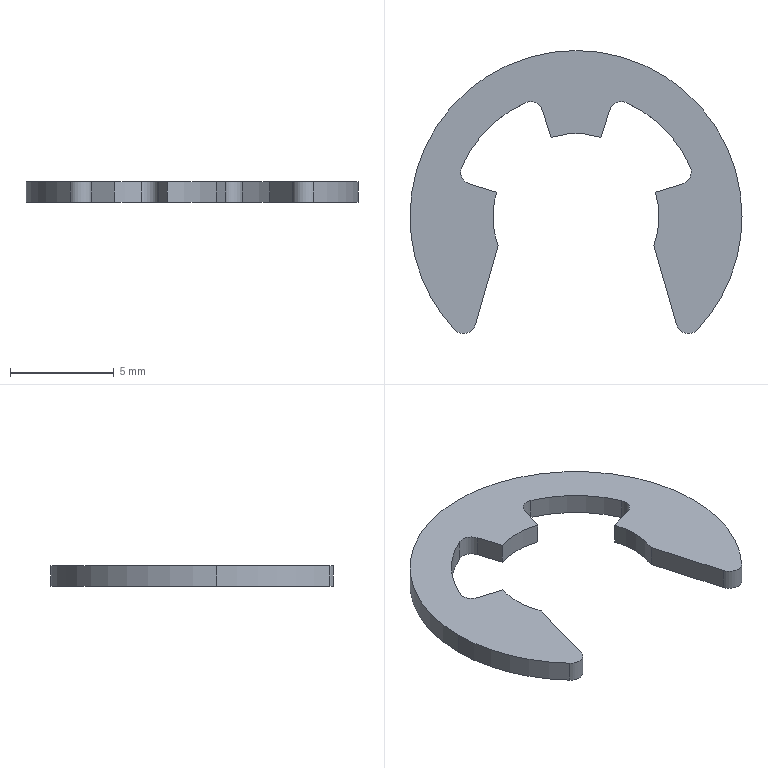Part | SolidWorks | features Extrusion 1 | 1 solid | 24 faces | box 16 x 13.638 x 1 mm | volume 90.427 mm3 | cylinder 16 | plane 8 | commonest cylinder face diameters 1.2 x7 8 x4 16 x3 12 x2
STEP:
#1=CARTESIAN_POINT('',(-5.507,2.381,1.));
#2=VERTEX_POINT('',#1);
#3=CARTESIAN_POINT('',(-5.557,2.143,1.));
#4=VERTEX_POINT('',#3);
#5=CARTESIAN_POINT('',(-4.957,2.143,1.));
#6=DIRECTION('',(0.,0.,1.));
#7=DIRECTION('',(1.,0.,0.));
#8=AXIS2_PLACEMENT_3D('',#5,#6,#7);
#9=CIRCLE('',#8,0.6);
#10=EDGE_CURVE('',#2,#4,#9,.T.);
#11=ORIENTED_EDGE('',*,*,#10,.T.);
#12=CARTESIAN_POINT('',(-5.557,2.143,0.));
#13=VERTEX_POINT('',#12);
#14=CARTESIAN_POINT('',(-5.557,2.143,1.));
#15=DIRECTION('',(0.,0.,-1.));
#16=VECTOR('',#15,1000.);
#17=LINE('',#14,#16);
#18=EDGE_CURVE('',#4,#13,#17,.T.);
#19=ORIENTED_EDGE('',*,*,#18,.T.);
#20=CARTESIAN_POINT('',(-5.507,2.381,0.));
#21=VERTEX_POINT('',#20);
#22=CARTESIAN_POINT('',(-4.957,2.143,0.));
#23=DIRECTION('',(0.,0.,1.));
#24=DIRECTION('',(1.,0.,0.));
#25=AXIS2_PLACEMENT_3D('',#22,#23,#24);
#26=CIRCLE('',#25,0.6);
#27=EDGE_CURVE('',#21,#13,#26,.T.);
#28=ORIENTED_EDGE('',*,*,#27,.F.);
#29=CARTESIAN_POINT('',(-5.507,2.381,1.));
#30=DIRECTION('',(0.,0.,-1.));
#31=VECTOR('',#30,1000.);
#32=LINE('',#29,#31);
#33=EDGE_CURVE('',#2,#21,#32,.T.);
#34=ORIENTED_EDGE('',*,*,#33,.F.);
#35=EDGE_LOOP('',(#11,#19,#28,#34));
#36=FACE_OUTER_BOUND('',#35,.T.);
#37=CARTESIAN_POINT('',(-4.957,2.143,1.));
#38=DIRECTION('',(0.,0.,-1.));
#39=DIRECTION('',(-1.,0.,0.));
#40=AXIS2_PLACEMENT_3D('',#37,#38,#39);
#41=CYLINDRICAL_SURFACE('',#40,0.6);
#42=ADVANCED_FACE('',(#36),#41,.F.);
#43=CARTESIAN_POINT('',(-3.825,1.169,1.));
#44=VERTEX_POINT('',#43);
#45=CARTESIAN_POINT('',(-4.,0.,1.));
#46=VERTEX_POINT('',#45);
#47=CARTESIAN_POINT('',(0.,0.,1.));
#48=DIRECTION('',(0.,0.,1.));
#49=DIRECTION('',(1.,0.,0.));
#50=AXIS2_PLACEMENT_3D('',#47,#48,#49);
#51=CIRCLE('',#50,4.);
#52=EDGE_CURVE('',#44,#46,#51,.T.);
#53=ORIENTED_EDGE('',*,*,#52,.T.);
#54=CARTESIAN_POINT('',(-4.,0.,0.));
#55=VERTEX_POINT('',#54);
#56=CARTESIAN_POINT('',(-4.,0.,1.));
#57=DIRECTION('',(0.,0.,-1.));
#58=VECTOR('',#57,1000.);
#59=LINE('',#56,#58);
#60=EDGE_CURVE('',#46,#55,#59,.T.);
#61=ORIENTED_EDGE('',*,*,#60,.T.);
#62=CARTESIAN_POINT('',(-3.825,1.169,0.));
#63=VERTEX_POINT('',#62);
#64=CARTESIAN_POINT('',(0.,0.,0.));
#65=DIRECTION('',(0.,0.,1.));
#66=DIRECTION('',(1.,0.,0.));
#67=AXIS2_PLACEMENT_3D('',#64,#65,#66);
#68=CIRCLE('',#67,4.);
#69=EDGE_CURVE('',#63,#55,#68,.T.);
#70=ORIENTED_EDGE('',*,*,#69,.F.);
#71=CARTESIAN_POINT('',(-3.825,1.169,1.));
#72=DIRECTION('',(0.,0.,-1.));
#73=VECTOR('',#72,1000.);
#74=LINE('',#71,#73);
#75=EDGE_CURVE('',#44,#63,#74,.T.);
#76=ORIENTED_EDGE('',*,*,#75,.F.);
#77=EDGE_LOOP('',(#53,#61,#70,#76));
#78=FACE_OUTER_BOUND('',#77,.T.);
#79=CARTESIAN_POINT('',(0.,0.,1.));
#80=DIRECTION('',(0.,0.,-1.));
#81=DIRECTION('',(-1.,0.,0.));
#82=AXIS2_PLACEMENT_3D('',#79,#80,#81);
#83=CYLINDRICAL_SURFACE('',#82,4.);
#84=ADVANCED_FACE('',(#78),#83,.F.);
#85=CARTESIAN_POINT('',(8.,0.,1.));
#86=VERTEX_POINT('',#85);
#87=CARTESIAN_POINT('',(-8.,0.,1.));
#88=VERTEX_POINT('',#87);
#89=CARTESIAN_POINT('',(0.,0.,1.));
#90=DIRECTION('',(0.,0.,1.));
#91=DIRECTION('',(1.,0.,0.));
#92=AXIS2_PLACEMENT_3D('',#89,#90,#91);
#93=CIRCLE('',#92,8.);
#94=EDGE_CURVE('',#86,#88,#93,.T.);
#95=ORIENTED_EDGE('',*,*,#94,.F.);
#96=CARTESIAN_POINT('',(8.,0.,0.));
#97=VERTEX_POINT('',#96);
#98=CARTESIAN_POINT('',(8.,0.,1.));
#99=DIRECTION('',(0.,0.,-1.));
#100=VECTOR('',#99,1000.);
#101=LINE('',#98,#100);
#102=EDGE_CURVE('',#86,#97,#101,.T.);
#103=ORIENTED_EDGE('',*,*,#102,.T.);
#104=CARTESIAN_POINT('',(-8.,0.,0.));
#105=VERTEX_POINT('',#104);
#106=CARTESIAN_POINT('',(0.,0.,0.));
#107=DIRECTION('',(0.,0.,1.));
#108=DIRECTION('',(1.,0.,0.));
#109=AXIS2_PLACEMENT_3D('',#106,#107,#108);
#110=CIRCLE('',#109,8.);
#111=EDGE_CURVE('',#97,#105,#110,.T.);
#112=ORIENTED_EDGE('',*,*,#111,.T.);
#113=CARTESIAN_POINT('',(-8.,0.,1.));
#114=DIRECTION('',(0.,0.,-1.));
#115=VECTOR('',#114,1000.);
#116=LINE('',#113,#115);
#117=EDGE_CURVE('',#88,#105,#116,.T.);
#118=ORIENTED_EDGE('',*,*,#117,.F.);
#119=EDGE_LOOP('',(#95,#103,#112,#118));
#120=FACE_OUTER_BOUND('',#119,.T.);
#121=CARTESIAN_POINT('',(0.,0.,1.));
#122=DIRECTION('',(0.,0.,-1.));
#123=DIRECTION('',(-1.,0.,0.));
#124=AXIS2_PLACEMENT_3D('',#121,#122,#123);
#125=CYLINDRICAL_SURFACE('',#124,8.);
#126=ADVANCED_FACE('',(#120),#125,.T.);
#127=CARTESIAN_POINT('',(-5.859,-5.447,1.));
#128=VERTEX_POINT('',#127);
#129=CARTESIAN_POINT('',(0.,0.,1.));
#130=DIRECTION('',(0.,0.,1.));
#131=DIRECTION('',(1.,0.,0.));
#132=AXIS2_PLACEMENT_3D('',#129,#130,#131);
#133=CIRCLE('',#132,8.);
#134=EDGE_CURVE('',#88,#128,#133,.T.);
#135=ORIENTED_EDGE('',*,*,#134,.F.);
#136=ORIENTED_EDGE('',*,*,#117,.T.);
#137=CARTESIAN_POINT('',(-5.859,-5.447,0.));
#138=VERTEX_POINT('',#137);
#139=CARTESIAN_POINT('',(0.,0.,0.));
#140=DIRECTION('',(0.,0.,1.));
#141=DIRECTION('',(1.,0.,0.));
#142=AXIS2_PLACEMENT_3D('',#139,#140,#141);
#143=CIRCLE('',#142,8.);
#144=EDGE_CURVE('',#105,#138,#143,.T.);
#145=ORIENTED_EDGE('',*,*,#144,.T.);
#146=CARTESIAN_POINT('',(-5.859,-5.447,1.));
#147=DIRECTION('',(0.,0.,-1.));
#148=VECTOR('',#147,1000.);
#149=LINE('',#146,#148);
#150=EDGE_CURVE('',#128,#138,#149,.T.);
#151=ORIENTED_EDGE('',*,*,#150,.F.);
#152=EDGE_LOOP('',(#135,#136,#145,#151));
#153=FACE_OUTER_BOUND('',#152,.T.);
#154=CARTESIAN_POINT('',(0.,0.,1.));
#155=DIRECTION('',(0.,0.,-1.));
#156=DIRECTION('',(-1.,0.,0.));
#157=AXIS2_PLACEMENT_3D('',#154,#155,#156);
#158=CYLINDRICAL_SURFACE('',#157,8.);
#159=ADVANCED_FACE('',(#153),#158,.T.);
#160=CARTESIAN_POINT('',(5.507,2.381,0.));
#161=VERTEX_POINT('',#160);
#162=CARTESIAN_POINT('',(2.429,5.486,0.));
#163=VERTEX_POINT('',#162);
#164=CARTESIAN_POINT('',(0.,0.,0.));
#165=DIRECTION('',(0.,0.,1.));
#166=DIRECTION('',(1.,0.,0.));
#167=AXIS2_PLACEMENT_3D('',#164,#165,#166);
#168=CIRCLE('',#167,6.);
#169=EDGE_CURVE('',#161,#163,#168,.T.);
#170=ORIENTED_EDGE('',*,*,#169,.F.);
#171=CARTESIAN_POINT('',(5.507,2.381,1.));
#172=VERTEX_POINT('',#171);
#173=CARTESIAN_POINT('',(5.507,2.381,1.));
#174=DIRECTION('',(0.,0.,-1.));
#175=VECTOR('',#174,1000.);
#176=LINE('',#173,#175);
#177=EDGE_CURVE('',#172,#161,#176,.T.);
#178=ORIENTED_EDGE('',*,*,#177,.F.);
#179=CARTESIAN_POINT('',(2.429,5.486,1.));
#180=VERTEX_POINT('',#179);
#181=CARTESIAN_POINT('',(0.,0.,1.));
#182=DIRECTION('',(0.,0.,1.));
#183=DIRECTION('',(1.,0.,0.));
#184=AXIS2_PLACEMENT_3D('',#181,#182,#183);
#185=CIRCLE('',#184,6.);
#186=EDGE_CURVE('',#172,#180,#185,.T.);
#187=ORIENTED_EDGE('',*,*,#186,.T.);
#188=CARTESIAN_POINT('',(2.429,5.486,1.));
#189=DIRECTION('',(0.,0.,-1.));
#190=VECTOR('',#189,1000.);
#191=LINE('',#188,#190);
#192=EDGE_CURVE('',#180,#163,#191,.T.);
#193=ORIENTED_EDGE('',*,*,#192,.T.);
#194=EDGE_LOOP('',(#170,#178,#187,#193));
#195=FACE_OUTER_BOUND('',#194,.T.);
#196=CARTESIAN_POINT('',(0.,0.,1.));
#197=DIRECTION('',(0.,0.,-1.));
#198=DIRECTION('',(-1.,0.,0.));
#199=AXIS2_PLACEMENT_3D('',#196,#197,#198);
#200=CYLINDRICAL_SURFACE('',#199,6.);
#201=ADVANCED_FACE('',(#195),#200,.F.);
#202=CARTESIAN_POINT('',(5.132,1.569,0.));
#203=VERTEX_POINT('',#202);
#204=CARTESIAN_POINT('',(4.957,2.143,0.));
#205=DIRECTION('',(0.,0.,-1.));
#206=DIRECTION('',(1.,0.,0.));
#207=AXIS2_PLACEMENT_3D('',#204,#205,#206);
#208=CIRCLE('',#207,0.6);
#209=EDGE_CURVE('',#161,#203,#208,.T.);
#210=ORIENTED_EDGE('',*,*,#209,.T.);
#211=CARTESIAN_POINT('',(5.132,1.569,1.));
#212=VERTEX_POINT('',#211);
#213=CARTESIAN_POINT('',(5.132,1.569,1.));
#214=DIRECTION('',(0.,0.,-1.));
#215=VECTOR('',#214,1000.);
#216=LINE('',#213,#215);
#217=EDGE_CURVE('',#212,#203,#216,.T.);
#218=ORIENTED_EDGE('',*,*,#217,.F.);
#219=CARTESIAN_POINT('',(4.957,2.143,1.));
#220=DIRECTION('',(0.,0.,-1.));
#221=DIRECTION('',(1.,0.,0.));
#222=AXIS2_PLACEMENT_3D('',#219,#220,#221);
#223=CIRCLE('',#222,0.6);
#224=EDGE_CURVE('',#172,#212,#223,.T.);
#225=ORIENTED_EDGE('',*,*,#224,.F.);
#226=ORIENTED_EDGE('',*,*,#177,.T.);
#227=EDGE_LOOP('',(#210,#218,#225,#226));
#228=FACE_OUTER_BOUND('',#227,.T.);
#229=CARTESIAN_POINT('',(4.957,2.143,1.));
#230=DIRECTION('',(0.,0.,-1.));
#231=DIRECTION('',(-1.,0.,0.));
#232=AXIS2_PLACEMENT_3D('',#229,#230,#231);
#233=CYLINDRICAL_SURFACE('',#232,0.6);
#234=ADVANCED_FACE('',(#228),#233,.F.);
#235=CARTESIAN_POINT('',(3.825,1.169,0.));
#236=VERTEX_POINT('',#235);
#237=CARTESIAN_POINT('',(0.,0.,0.));
#238=DIRECTION('',(0.9563,0.2924,0.));
#239=VECTOR('',#238,1000.);
#240=LINE('',#237,#239);
#241=EDGE_CURVE('',#236,#203,#240,.T.);
#242=ORIENTED_EDGE('',*,*,#241,.F.);
#243=CARTESIAN_POINT('',(3.825,1.169,1.));
#244=VERTEX_POINT('',#243);
#245=CARTESIAN_POINT('',(3.825,1.169,1.));
#246=DIRECTION('',(0.,0.,-1.));
#247=VECTOR('',#246,1000.);
#248=LINE('',#245,#247);
#249=EDGE_CURVE('',#244,#236,#248,.T.);
#250=ORIENTED_EDGE('',*,*,#249,.F.);
#251=CARTESIAN_POINT('',(0.,0.,1.));
#252=DIRECTION('',(0.9563,0.2924,0.));
#253=VECTOR('',#252,1000.);
#254=LINE('',#251,#253);
#255=EDGE_CURVE('',#244,#212,#254,.T.);
#256=ORIENTED_EDGE('',*,*,#255,.T.);
#257=ORIENTED_EDGE('',*,*,#217,.T.);
#258=EDGE_LOOP('',(#242,#250,#256,#257));
#259=FACE_OUTER_BOUND('',#258,.T.);
#260=CARTESIAN_POINT('',(0.,0.,1.));
#261=DIRECTION('',(-0.2924,0.9563,0.));
#262=DIRECTION('',(-0.9563,-0.2924,0.));
#263=AXIS2_PLACEMENT_3D('',#260,#261,#262);
#264=PLANE('',#263);
#265=ADVANCED_FACE('',(#259),#264,.T.);
#266=CARTESIAN_POINT('',(3.75,-1.392,0.));
#267=VERTEX_POINT('',#266);
#268=CARTESIAN_POINT('',(0.,0.,0.));
#269=DIRECTION('',(0.,0.,1.));
#270=DIRECTION('',(1.,0.,0.));
#271=AXIS2_PLACEMENT_3D('',#268,#269,#270);
#272=CIRCLE('',#271,4.);
#273=EDGE_CURVE('',#267,#236,#272,.T.);
#274=ORIENTED_EDGE('',*,*,#273,.F.);
#275=CARTESIAN_POINT('',(3.75,-1.392,1.));
#276=VERTEX_POINT('',#275);
#277=CARTESIAN_POINT('',(3.75,-1.392,1.));
#278=DIRECTION('',(0.,0.,-1.));
#279=VECTOR('',#278,1000.);
#280=LINE('',#277,#279);
#281=EDGE_CURVE('',#276,#267,#280,.T.);
#282=ORIENTED_EDGE('',*,*,#281,.F.);
#283=CARTESIAN_POINT('',(0.,0.,1.));
#284=DIRECTION('',(0.,0.,1.));
#285=DIRECTION('',(1.,0.,0.));
#286=AXIS2_PLACEMENT_3D('',#283,#284,#285);
#287=CIRCLE('',#286,4.);
#288=EDGE_CURVE('',#276,#244,#287,.T.);
#289=ORIENTED_EDGE('',*,*,#288,.T.);
#290=ORIENTED_EDGE('',*,*,#249,.T.);
#291=EDGE_LOOP('',(#274,#282,#289,#290));
#292=FACE_OUTER_BOUND('',#291,.T.);
#293=CARTESIAN_POINT('',(0.,0.,1.));
#294=DIRECTION('',(0.,0.,-1.));
#295=DIRECTION('',(-1.,0.,0.));
#296=AXIS2_PLACEMENT_3D('',#293,#294,#295);
#297=CYLINDRICAL_SURFACE('',#296,4.);
#298=ADVANCED_FACE('',(#292),#297,.F.);
#299=CARTESIAN_POINT('',(4.843,-5.204,0.));
#300=VERTEX_POINT('',#299);
#301=CARTESIAN_POINT('',(3.096,0.8878,0.));
#302=DIRECTION('',(0.2756,-0.9613,0.));
#303=VECTOR('',#302,1000.);
#304=LINE('',#301,#303);
#305=EDGE_CURVE('',#267,#300,#304,.T.);
#306=ORIENTED_EDGE('',*,*,#305,.T.);
#307=CARTESIAN_POINT('',(4.843,-5.204,1.));
#308=VERTEX_POINT('',#307);
#309=CARTESIAN_POINT('',(4.843,-5.204,1.));
#310=DIRECTION('',(0.,0.,-1.));
#311=VECTOR('',#310,1000.);
#312=LINE('',#309,#311);
#313=EDGE_CURVE('',#308,#300,#312,.T.);
#314=ORIENTED_EDGE('',*,*,#313,.F.);
#315=CARTESIAN_POINT('',(3.096,0.8878,1.));
#316=DIRECTION('',(0.2756,-0.9613,0.));
#317=VECTOR('',#316,1000.);
#318=LINE('',#315,#317);
#319=EDGE_CURVE('',#276,#308,#318,.T.);
#320=ORIENTED_EDGE('',*,*,#319,.F.);
#321=ORIENTED_EDGE('',*,*,#281,.T.);
#322=EDGE_LOOP('',(#306,#314,#320,#321));
#323=FACE_OUTER_BOUND('',#322,.T.);
#324=CARTESIAN_POINT('',(3.096,0.8878,1.));
#325=DIRECTION('',(0.9613,0.2756,0.));
#326=DIRECTION('',(-0.2756,0.9613,0.));
#327=AXIS2_PLACEMENT_3D('',#324,#325,#326);
#328=PLANE('',#327);
#329=ADVANCED_FACE('',(#323),#328,.F.);
#330=CARTESIAN_POINT('',(5.859,-5.447,0.));
#331=VERTEX_POINT('',#330);
#332=CARTESIAN_POINT('',(5.42,-5.038,0.));
#333=DIRECTION('',(0.,0.,-1.));
#334=DIRECTION('',(1.,0.,0.));
#335=AXIS2_PLACEMENT_3D('',#332,#333,#334);
#336=CIRCLE('',#335,0.6);
#337=EDGE_CURVE('',#331,#300,#336,.T.);
#338=ORIENTED_EDGE('',*,*,#337,.F.);
#339=CARTESIAN_POINT('',(5.859,-5.447,1.));
#340=VERTEX_POINT('',#339);
#341=CARTESIAN_POINT('',(5.859,-5.447,1.));
#342=DIRECTION('',(0.,0.,-1.));
#343=VECTOR('',#342,1000.);
#344=LINE('',#341,#343);
#345=EDGE_CURVE('',#340,#331,#344,.T.);
#346=ORIENTED_EDGE('',*,*,#345,.F.);
#347=CARTESIAN_POINT('',(5.42,-5.038,1.));
#348=DIRECTION('',(0.,0.,-1.));
#349=DIRECTION('',(1.,0.,0.));
#350=AXIS2_PLACEMENT_3D('',#347,#348,#349);
#351=CIRCLE('',#350,0.6);
#352=EDGE_CURVE('',#340,#308,#351,.T.);
#353=ORIENTED_EDGE('',*,*,#352,.T.);
#354=ORIENTED_EDGE('',*,*,#313,.T.);
#355=EDGE_LOOP('',(#338,#346,#353,#354));
#356=FACE_OUTER_BOUND('',#355,.T.);
#357=CARTESIAN_POINT('',(5.42,-5.038,1.));
#358=DIRECTION('',(0.,0.,-1.));
#359=DIRECTION('',(-1.,0.,0.));
#360=AXIS2_PLACEMENT_3D('',#357,#358,#359);
#361=CYLINDRICAL_SURFACE('',#360,0.6);
#362=ADVANCED_FACE('',(#356),#361,.T.);
#363=ORIENTED_EDGE('',*,*,#102,.F.);
#364=CARTESIAN_POINT('',(0.,0.,1.));
#365=DIRECTION('',(0.,0.,1.));
#366=DIRECTION('',(1.,0.,0.));
#367=AXIS2_PLACEMENT_3D('',#364,#365,#366);
#368=CIRCLE('',#367,8.);
#369=EDGE_CURVE('',#340,#86,#368,.T.);
#370=ORIENTED_EDGE('',*,*,#369,.F.);
#371=ORIENTED_EDGE('',*,*,#345,.T.);
#372=CARTESIAN_POINT('',(0.,0.,0.));
#373=DIRECTION('',(0.,0.,1.));
#374=DIRECTION('',(1.,0.,0.));
#375=AXIS2_PLACEMENT_3D('',#372,#373,#374);
#376=CIRCLE('',#375,8.);
#377=EDGE_CURVE('',#331,#97,#376,.T.);
#378=ORIENTED_EDGE('',*,*,#377,.T.);
#379=EDGE_LOOP('',(#363,#370,#371,#378));
#380=FACE_OUTER_BOUND('',#379,.T.);
#381=CARTESIAN_POINT('',(0.,0.,1.));
#382=DIRECTION('',(0.,0.,-1.));
#383=DIRECTION('',(-1.,0.,0.));
#384=AXIS2_PLACEMENT_3D('',#381,#382,#383);
#385=CYLINDRICAL_SURFACE('',#384,8.);
#386=ADVANCED_FACE('',(#380),#385,.T.);
#387=CARTESIAN_POINT('',(-4.843,-5.204,0.));
#388=VERTEX_POINT('',#387);
#389=CARTESIAN_POINT('',(-5.42,-5.038,0.));
#390=DIRECTION('',(0.,0.,-1.));
#391=DIRECTION('',(1.,0.,0.));
#392=AXIS2_PLACEMENT_3D('',#389,#390,#391);
#393=CIRCLE('',#392,0.6);
#394=EDGE_CURVE('',#388,#138,#393,.T.);
#395=ORIENTED_EDGE('',*,*,#394,.F.);
#396=CARTESIAN_POINT('',(-4.843,-5.204,1.));
#397=VERTEX_POINT('',#396);
#398=CARTESIAN_POINT('',(-4.843,-5.204,1.));
#399=DIRECTION('',(0.,0.,-1.));
#400=VECTOR('',#399,1000.);
#401=LINE('',#398,#400);
#402=EDGE_CURVE('',#397,#388,#401,.T.);
#403=ORIENTED_EDGE('',*,*,#402,.F.);
#404=CARTESIAN_POINT('',(-5.42,-5.038,1.));
#405=DIRECTION('',(0.,0.,-1.));
#406=DIRECTION('',(1.,0.,0.));
#407=AXIS2_PLACEMENT_3D('',#404,#405,#406);
#408=CIRCLE('',#407,0.6);
#409=EDGE_CURVE('',#397,#128,#408,.T.);
#410=ORIENTED_EDGE('',*,*,#409,.T.);
#411=ORIENTED_EDGE('',*,*,#150,.T.);
#412=EDGE_LOOP('',(#395,#403,#410,#411));
#413=FACE_OUTER_BOUND('',#412,.T.);
#414=CARTESIAN_POINT('',(-5.42,-5.038,1.));
#415=DIRECTION('',(0.,0.,-1.));
#416=DIRECTION('',(-1.,0.,0.));
#417=AXIS2_PLACEMENT_3D('',#414,#415,#416);
#418=CYLINDRICAL_SURFACE('',#417,0.6);
#419=ADVANCED_FACE('',(#413),#418,.T.);
#420=CARTESIAN_POINT('',(-3.75,-1.392,0.));
#421=VERTEX_POINT('',#420);
#422=CARTESIAN_POINT('',(-3.096,0.8878,0.));
#423=DIRECTION('',(-0.2756,-0.9613,0.));
#424=VECTOR('',#423,1000.);
#425=LINE('',#422,#424);
#426=EDGE_CURVE('',#421,#388,#425,.T.);
#427=ORIENTED_EDGE('',*,*,#426,.F.);
#428=CARTESIAN_POINT('',(-3.75,-1.392,1.));
#429=VERTEX_POINT('',#428);
#430=CARTESIAN_POINT('',(-3.75,-1.392,1.));
#431=DIRECTION('',(0.,0.,-1.));
#432=VECTOR('',#431,1000.);
#433=LINE('',#430,#432);
#434=EDGE_CURVE('',#429,#421,#433,.T.);
#435=ORIENTED_EDGE('',*,*,#434,.F.);
#436=CARTESIAN_POINT('',(-3.096,0.8878,1.));
#437=DIRECTION('',(-0.2756,-0.9613,0.));
#438=VECTOR('',#437,1000.);
#439=LINE('',#436,#438);
#440=EDGE_CURVE('',#429,#397,#439,.T.);
#441=ORIENTED_EDGE('',*,*,#440,.T.);
#442=ORIENTED_EDGE('',*,*,#402,.T.);
#443=EDGE_LOOP('',(#427,#435,#441,#442));
#444=FACE_OUTER_BOUND('',#443,.T.);
#445=CARTESIAN_POINT('',(-3.096,0.8878,1.));
#446=DIRECTION('',(0.9613,-0.2756,0.));
#447=DIRECTION('',(0.2756,0.9613,0.));
#448=AXIS2_PLACEMENT_3D('',#445,#446,#447);
#449=PLANE('',#448);
#450=ADVANCED_FACE('',(#444),#449,.T.);
#451=ORIENTED_EDGE('',*,*,#60,.F.);
#452=CARTESIAN_POINT('',(0.,0.,1.));
#453=DIRECTION('',(0.,0.,1.));
#454=DIRECTION('',(1.,0.,0.));
#455=AXIS2_PLACEMENT_3D('',#452,#453,#454);
#456=CIRCLE('',#455,4.);
#457=EDGE_CURVE('',#46,#429,#456,.T.);
#458=ORIENTED_EDGE('',*,*,#457,.T.);
#459=ORIENTED_EDGE('',*,*,#434,.T.);
#460=CARTESIAN_POINT('',(0.,0.,0.));
#461=DIRECTION('',(0.,0.,1.));
#462=DIRECTION('',(1.,0.,0.));
#463=AXIS2_PLACEMENT_3D('',#460,#461,#462);
#464=CIRCLE('',#463,4.);
#465=EDGE_CURVE('',#55,#421,#464,.T.);
#466=ORIENTED_EDGE('',*,*,#465,.F.);
#467=EDGE_LOOP('',(#451,#458,#459,#466));
#468=FACE_OUTER_BOUND('',#467,.T.);
#469=CARTESIAN_POINT('',(0.,0.,1.));
#470=DIRECTION('',(0.,0.,-1.));
#471=DIRECTION('',(-1.,0.,0.));
#472=AXIS2_PLACEMENT_3D('',#469,#470,#471);
#473=CYLINDRICAL_SURFACE('',#472,4.);
#474=ADVANCED_FACE('',(#468),#473,.F.);
#475=CARTESIAN_POINT('',(-5.132,1.569,0.));
#476=VERTEX_POINT('',#475);
#477=CARTESIAN_POINT('',(0.,0.,0.));
#478=DIRECTION('',(-0.9563,0.2924,0.));
#479=VECTOR('',#478,1000.);
#480=LINE('',#477,#479);
#481=EDGE_CURVE('',#63,#476,#480,.T.);
#482=ORIENTED_EDGE('',*,*,#481,.T.);
#483=CARTESIAN_POINT('',(-5.132,1.569,1.));
#484=VERTEX_POINT('',#483);
#485=CARTESIAN_POINT('',(-5.132,1.569,1.));
#486=DIRECTION('',(0.,0.,-1.));
#487=VECTOR('',#486,1000.);
#488=LINE('',#485,#487);
#489=EDGE_CURVE('',#484,#476,#488,.T.);
#490=ORIENTED_EDGE('',*,*,#489,.F.);
#491=CARTESIAN_POINT('',(0.,0.,1.));
#492=DIRECTION('',(-0.9563,0.2924,0.));
#493=VECTOR('',#492,1000.);
#494=LINE('',#491,#493);
#495=EDGE_CURVE('',#44,#484,#494,.T.);
#496=ORIENTED_EDGE('',*,*,#495,.F.);
#497=ORIENTED_EDGE('',*,*,#75,.T.);
#498=EDGE_LOOP('',(#482,#490,#496,#497));
#499=FACE_OUTER_BOUND('',#498,.T.);
#500=CARTESIAN_POINT('',(0.,0.,1.));
#501=DIRECTION('',(-0.2924,-0.9563,0.));
#502=DIRECTION('',(0.9563,-0.2924,0.));
#503=AXIS2_PLACEMENT_3D('',#500,#501,#502);
#504=PLANE('',#503);
#505=ADVANCED_FACE('',(#499),#504,.F.);
#506=ORIENTED_EDGE('',*,*,#18,.F.);
#507=CARTESIAN_POINT('',(-4.957,2.143,1.));
#508=DIRECTION('',(0.,0.,1.));
#509=DIRECTION('',(1.,0.,0.));
#510=AXIS2_PLACEMENT_3D('',#507,#508,#509);
#511=CIRCLE('',#510,0.6);
#512=EDGE_CURVE('',#4,#484,#511,.T.);
#513=ORIENTED_EDGE('',*,*,#512,.T.);
#514=ORIENTED_EDGE('',*,*,#489,.T.);
#515=CARTESIAN_POINT('',(-4.957,2.143,0.));
#516=DIRECTION('',(0.,0.,1.));
#517=DIRECTION('',(1.,0.,0.));
#518=AXIS2_PLACEMENT_3D('',#515,#516,#517);
#519=CIRCLE('',#518,0.6);
#520=EDGE_CURVE('',#13,#476,#519,.T.);
#521=ORIENTED_EDGE('',*,*,#520,.F.);
#522=EDGE_LOOP('',(#506,#513,#514,#521));
#523=FACE_OUTER_BOUND('',#522,.T.);
#524=CARTESIAN_POINT('',(-4.957,2.143,1.));
#525=DIRECTION('',(0.,0.,-1.));
#526=DIRECTION('',(-1.,0.,0.));
#527=AXIS2_PLACEMENT_3D('',#524,#525,#526);
#528=CYLINDRICAL_SURFACE('',#527,0.6);
#529=ADVANCED_FACE('',(#523),#528,.F.);
#530=CARTESIAN_POINT('',(-2.429,5.486,0.));
#531=VERTEX_POINT('',#530);
#532=CARTESIAN_POINT('',(0.,0.,0.));
#533=DIRECTION('',(0.,0.,1.));
#534=DIRECTION('',(1.,0.,0.));
#535=AXIS2_PLACEMENT_3D('',#532,#533,#534);
#536=CIRCLE('',#535,6.);
#537=EDGE_CURVE('',#531,#21,#536,.T.);
#538=ORIENTED_EDGE('',*,*,#537,.F.);
#539=CARTESIAN_POINT('',(-2.429,5.486,1.));
#540=VERTEX_POINT('',#539);
#541=CARTESIAN_POINT('',(-2.429,5.486,1.));
#542=DIRECTION('',(0.,0.,-1.));
#543=VECTOR('',#542,1000.);
#544=LINE('',#541,#543);
#545=EDGE_CURVE('',#540,#531,#544,.T.);
#546=ORIENTED_EDGE('',*,*,#545,.F.);
#547=CARTESIAN_POINT('',(0.,0.,1.));
#548=DIRECTION('',(0.,0.,1.));
#549=DIRECTION('',(1.,0.,0.));
#550=AXIS2_PLACEMENT_3D('',#547,#548,#549);
#551=CIRCLE('',#550,6.);
#552=EDGE_CURVE('',#540,#2,#551,.T.);
#553=ORIENTED_EDGE('',*,*,#552,.T.);
#554=ORIENTED_EDGE('',*,*,#33,.T.);
#555=EDGE_LOOP('',(#538,#546,#553,#554));
#556=FACE_OUTER_BOUND('',#555,.T.);
#557=CARTESIAN_POINT('',(0.,0.,1.));
#558=DIRECTION('',(0.,0.,-1.));
#559=DIRECTION('',(-1.,0.,0.));
#560=AXIS2_PLACEMENT_3D('',#557,#558,#559);
#561=CYLINDRICAL_SURFACE('',#560,6.);
#562=ADVANCED_FACE('',(#556),#561,.F.);
#563=CARTESIAN_POINT('',(-1.614,5.118,0.));
#564=VERTEX_POINT('',#563);
#565=CARTESIAN_POINT('',(-2.186,4.938,0.));
#566=DIRECTION('',(0.,0.,1.));
#567=DIRECTION('',(1.,0.,0.));
#568=AXIS2_PLACEMENT_3D('',#565,#566,#567);
#569=CIRCLE('',#568,0.6);
#570=EDGE_CURVE('',#564,#531,#569,.T.);
#571=ORIENTED_EDGE('',*,*,#570,.F.);
#572=CARTESIAN_POINT('',(-1.614,5.118,1.));
#573=VERTEX_POINT('',#572);
#574=CARTESIAN_POINT('',(-1.614,5.118,1.));
#575=DIRECTION('',(0.,0.,-1.));
#576=VECTOR('',#575,1000.);
#577=LINE('',#574,#576);
#578=EDGE_CURVE('',#573,#564,#577,.T.);
#579=ORIENTED_EDGE('',*,*,#578,.F.);
#580=CARTESIAN_POINT('',(-2.186,4.938,1.));
#581=DIRECTION('',(0.,0.,1.));
#582=DIRECTION('',(1.,0.,0.));
#583=AXIS2_PLACEMENT_3D('',#580,#581,#582);
#584=CIRCLE('',#583,0.6);
#585=EDGE_CURVE('',#573,#540,#584,.T.);
#586=ORIENTED_EDGE('',*,*,#585,.T.);
#587=ORIENTED_EDGE('',*,*,#545,.T.);
#588=EDGE_LOOP('',(#571,#579,#586,#587));
#589=FACE_OUTER_BOUND('',#588,.T.);
#590=CARTESIAN_POINT('',(-2.186,4.938,1.));
#591=DIRECTION('',(0.,0.,-1.));
#592=DIRECTION('',(-1.,0.,0.));
#593=AXIS2_PLACEMENT_3D('',#590,#591,#592);
#594=CYLINDRICAL_SURFACE('',#593,0.6);
#595=ADVANCED_FACE('',(#589),#594,.F.);
#596=CARTESIAN_POINT('',(-1.203,3.815,0.));
#597=VERTEX_POINT('',#596);
#598=CARTESIAN_POINT('',(0.,0.,0.));
#599=DIRECTION('',(-0.3007,0.9537,0.));
#600=VECTOR('',#599,1000.);
#601=LINE('',#598,#600);
#602=EDGE_CURVE('',#597,#564,#601,.T.);
#603=ORIENTED_EDGE('',*,*,#602,.F.);
#604=CARTESIAN_POINT('',(-1.203,3.815,1.));
#605=VERTEX_POINT('',#604);
#606=CARTESIAN_POINT('',(-1.203,3.815,1.));
#607=DIRECTION('',(0.,0.,-1.));
#608=VECTOR('',#607,1000.);
#609=LINE('',#606,#608);
#610=EDGE_CURVE('',#605,#597,#609,.T.);
#611=ORIENTED_EDGE('',*,*,#610,.F.);
#612=CARTESIAN_POINT('',(0.,0.,1.));
#613=DIRECTION('',(-0.3007,0.9537,0.));
#614=VECTOR('',#613,1000.);
#615=LINE('',#612,#614);
#616=EDGE_CURVE('',#605,#573,#615,.T.);
#617=ORIENTED_EDGE('',*,*,#616,.T.);
#618=ORIENTED_EDGE('',*,*,#578,.T.);
#619=EDGE_LOOP('',(#603,#611,#617,#618));
#620=FACE_OUTER_BOUND('',#619,.T.);
#621=CARTESIAN_POINT('',(0.,0.,1.));
#622=DIRECTION('',(-0.9537,-0.3007,0.));
#623=DIRECTION('',(0.3007,-0.9537,0.));
#624=AXIS2_PLACEMENT_3D('',#621,#622,#623);
#625=PLANE('',#624);
#626=ADVANCED_FACE('',(#620),#625,.T.);
#627=CARTESIAN_POINT('',(1.203,3.815,0.));
#628=VERTEX_POINT('',#627);
#629=CARTESIAN_POINT('',(0.,0.,0.));
#630=DIRECTION('',(0.,0.,1.));
#631=DIRECTION('',(1.,0.,0.));
#632=AXIS2_PLACEMENT_3D('',#629,#630,#631);
#633=CIRCLE('',#632,4.);
#634=EDGE_CURVE('',#628,#597,#633,.T.);
#635=ORIENTED_EDGE('',*,*,#634,.F.);
#636=CARTESIAN_POINT('',(1.203,3.815,1.));
#637=VERTEX_POINT('',#636);
#638=CARTESIAN_POINT('',(1.203,3.815,1.));
#639=DIRECTION('',(0.,0.,-1.));
#640=VECTOR('',#639,1000.);
#641=LINE('',#638,#640);
#642=EDGE_CURVE('',#637,#628,#641,.T.);
#643=ORIENTED_EDGE('',*,*,#642,.F.);
#644=CARTESIAN_POINT('',(0.,0.,1.));
#645=DIRECTION('',(0.,0.,1.));
#646=DIRECTION('',(1.,0.,0.));
#647=AXIS2_PLACEMENT_3D('',#644,#645,#646);
#648=CIRCLE('',#647,4.);
#649=EDGE_CURVE('',#637,#605,#648,.T.);
#650=ORIENTED_EDGE('',*,*,#649,.T.);
#651=ORIENTED_EDGE('',*,*,#610,.T.);
#652=EDGE_LOOP('',(#635,#643,#650,#651));
#653=FACE_OUTER_BOUND('',#652,.T.);
#654=CARTESIAN_POINT('',(0.,0.,1.));
#655=DIRECTION('',(0.,0.,-1.));
#656=DIRECTION('',(-1.,0.,0.));
#657=AXIS2_PLACEMENT_3D('',#654,#655,#656);
#658=CYLINDRICAL_SURFACE('',#657,4.);
#659=ADVANCED_FACE('',(#653),#658,.F.);
#660=CARTESIAN_POINT('',(1.614,5.118,0.));
#661=VERTEX_POINT('',#660);
#662=CARTESIAN_POINT('',(0.,0.,0.));
#663=DIRECTION('',(0.3007,0.9537,0.));
#664=VECTOR('',#663,1000.);
#665=LINE('',#662,#664);
#666=EDGE_CURVE('',#628,#661,#665,.T.);
#667=ORIENTED_EDGE('',*,*,#666,.T.);
#668=CARTESIAN_POINT('',(1.614,5.118,1.));
#669=VERTEX_POINT('',#668);
#670=CARTESIAN_POINT('',(1.614,5.118,1.));
#671=DIRECTION('',(0.,0.,-1.));
#672=VECTOR('',#671,1000.);
#673=LINE('',#670,#672);
#674=EDGE_CURVE('',#669,#661,#673,.T.);
#675=ORIENTED_EDGE('',*,*,#674,.F.);
#676=CARTESIAN_POINT('',(0.,0.,1.));
#677=DIRECTION('',(0.3007,0.9537,0.));
#678=VECTOR('',#677,1000.);
#679=LINE('',#676,#678);
#680=EDGE_CURVE('',#637,#669,#679,.T.);
#681=ORIENTED_EDGE('',*,*,#680,.F.);
#682=ORIENTED_EDGE('',*,*,#642,.T.);
#683=EDGE_LOOP('',(#667,#675,#681,#682));
#684=FACE_OUTER_BOUND('',#683,.T.);
#685=CARTESIAN_POINT('',(0.,0.,1.));
#686=DIRECTION('',(-0.9537,0.3007,0.));
#687=DIRECTION('',(-0.3007,-0.9537,0.));
#688=AXIS2_PLACEMENT_3D('',#685,#686,#687);
#689=PLANE('',#688);
#690=ADVANCED_FACE('',(#684),#689,.F.);
#691=CARTESIAN_POINT('',(2.186,4.938,0.));
#692=DIRECTION('',(0.,0.,1.));
#693=DIRECTION('',(1.,0.,0.));
#694=AXIS2_PLACEMENT_3D('',#691,#692,#693);
#695=CIRCLE('',#694,0.6);
#696=EDGE_CURVE('',#163,#661,#695,.T.);
#697=ORIENTED_EDGE('',*,*,#696,.F.);
#698=ORIENTED_EDGE('',*,*,#192,.F.);
#699=CARTESIAN_POINT('',(2.186,4.938,1.));
#700=DIRECTION('',(0.,0.,1.));
#701=DIRECTION('',(1.,0.,0.));
#702=AXIS2_PLACEMENT_3D('',#699,#700,#701);
#703=CIRCLE('',#702,0.6);
#704=EDGE_CURVE('',#180,#669,#703,.T.);
#705=ORIENTED_EDGE('',*,*,#704,.T.);
#706=ORIENTED_EDGE('',*,*,#674,.T.);
#707=EDGE_LOOP('',(#697,#698,#705,#706));
#708=FACE_OUTER_BOUND('',#707,.T.);
#709=CARTESIAN_POINT('',(2.186,4.938,1.));
#710=DIRECTION('',(0.,0.,-1.));
#711=DIRECTION('',(-1.,0.,0.));
#712=AXIS2_PLACEMENT_3D('',#709,#710,#711);
#713=CYLINDRICAL_SURFACE('',#712,0.6);
#714=ADVANCED_FACE('',(#708),#713,.F.);
#715=ORIENTED_EDGE('',*,*,#186,.F.);
#716=ORIENTED_EDGE('',*,*,#224,.T.);
#717=ORIENTED_EDGE('',*,*,#255,.F.);
#718=ORIENTED_EDGE('',*,*,#288,.F.);
#719=ORIENTED_EDGE('',*,*,#319,.T.);
#720=ORIENTED_EDGE('',*,*,#352,.F.);
#721=ORIENTED_EDGE('',*,*,#369,.T.);
#722=ORIENTED_EDGE('',*,*,#94,.T.);
#723=ORIENTED_EDGE('',*,*,#134,.T.);
#724=ORIENTED_EDGE('',*,*,#409,.F.);
#725=ORIENTED_EDGE('',*,*,#440,.F.);
#726=ORIENTED_EDGE('',*,*,#457,.F.);
#727=ORIENTED_EDGE('',*,*,#52,.F.);
#728=ORIENTED_EDGE('',*,*,#495,.T.);
#729=ORIENTED_EDGE('',*,*,#512,.F.);
#730=ORIENTED_EDGE('',*,*,#10,.F.);
#731=ORIENTED_EDGE('',*,*,#552,.F.);
#732=ORIENTED_EDGE('',*,*,#585,.F.);
#733=ORIENTED_EDGE('',*,*,#616,.F.);
#734=ORIENTED_EDGE('',*,*,#649,.F.);
#735=ORIENTED_EDGE('',*,*,#680,.T.);
#736=ORIENTED_EDGE('',*,*,#704,.F.);
#737=EDGE_LOOP('',(#715,#716,#717,#718,#719,#720,#721,#722,#723,#724,#725,#726,#727,#728,#729,#730,#731,#732,#733,#734,#735,#736));
#738=FACE_OUTER_BOUND('',#737,.T.);
#739=CARTESIAN_POINT('',(0.,0.,1.));
#740=DIRECTION('',(0.,0.,1.));
#741=DIRECTION('',(1.,0.,0.));
#742=AXIS2_PLACEMENT_3D('',#739,#740,#741);
#743=PLANE('',#742);
#744=ADVANCED_FACE('',(#738),#743,.T.);
#745=ORIENTED_EDGE('',*,*,#169,.T.);
#746=ORIENTED_EDGE('',*,*,#696,.T.);
#747=ORIENTED_EDGE('',*,*,#666,.F.);
#748=ORIENTED_EDGE('',*,*,#634,.T.);
#749=ORIENTED_EDGE('',*,*,#602,.T.);
#750=ORIENTED_EDGE('',*,*,#570,.T.);
#751=ORIENTED_EDGE('',*,*,#537,.T.);
#752=ORIENTED_EDGE('',*,*,#27,.T.);
#753=ORIENTED_EDGE('',*,*,#520,.T.);
#754=ORIENTED_EDGE('',*,*,#481,.F.);
#755=ORIENTED_EDGE('',*,*,#69,.T.);
#756=ORIENTED_EDGE('',*,*,#465,.T.);
#757=ORIENTED_EDGE('',*,*,#426,.T.);
#758=ORIENTED_EDGE('',*,*,#394,.T.);
#759=ORIENTED_EDGE('',*,*,#144,.F.);
#760=ORIENTED_EDGE('',*,*,#111,.F.);
#761=ORIENTED_EDGE('',*,*,#377,.F.);
#762=ORIENTED_EDGE('',*,*,#337,.T.);
#763=ORIENTED_EDGE('',*,*,#305,.F.);
#764=ORIENTED_EDGE('',*,*,#273,.T.);
#765=ORIENTED_EDGE('',*,*,#241,.T.);
#766=ORIENTED_EDGE('',*,*,#209,.F.);
#767=EDGE_LOOP('',(#745,#746,#747,#748,#749,#750,#751,#752,#753,#754,#755,#756,#757,#758,#759,#760,#761,#762,#763,#764,#765,#766));
#768=FACE_OUTER_BOUND('',#767,.T.);
#769=CARTESIAN_POINT('',(0.,0.,0.));
#770=DIRECTION('',(0.,0.,1.));
#771=DIRECTION('',(1.,0.,0.));
#772=AXIS2_PLACEMENT_3D('',#769,#770,#771);
#773=PLANE('',#772);
#774=ADVANCED_FACE('',(#768),#773,.F.);
#775=CLOSED_SHELL('',(#42,#84,#126,#159,#201,#234,#265,#298,#329,#362,#386,#419,#450,#474,#505,#529,#562,#595,#626,#659,#690,#714,#744,#774));
#776=MANIFOLD_SOLID_BREP('',#775);
#777=CARTESIAN_POINT('',(0.,0.,0.));
#778=DIRECTION('',(0.,0.,1.));
#779=DIRECTION('',(1.,0.,0.));
#780=AXIS2_PLACEMENT_3D('',#777,#778,#779);
#781=(LENGTH_UNIT()NAMED_UNIT(*)SI_UNIT(.MILLI.,.METRE.));
#782=UNCERTAINTY_MEASURE_WITH_UNIT(LENGTH_MEASURE(0.00001),#781,'','');
#783=(NAMED_UNIT(*)PLANE_ANGLE_UNIT()SI_UNIT($,.RADIAN.));
#784=(NAMED_UNIT(*)SI_UNIT($,.STERADIAN.)SOLID_ANGLE_UNIT());
#785=(GEOMETRIC_REPRESENTATION_CONTEXT(3)GLOBAL_UNCERTAINTY_ASSIGNED_CONTEXT((#782))GLOBAL_UNIT_ASSIGNED_CONTEXT((#781,#783,#784))REPRESENTATION_CONTEXT('',''));
#786=ADVANCED_BREP_SHAPE_REPRESENTATION('',(#776,#780),#785);